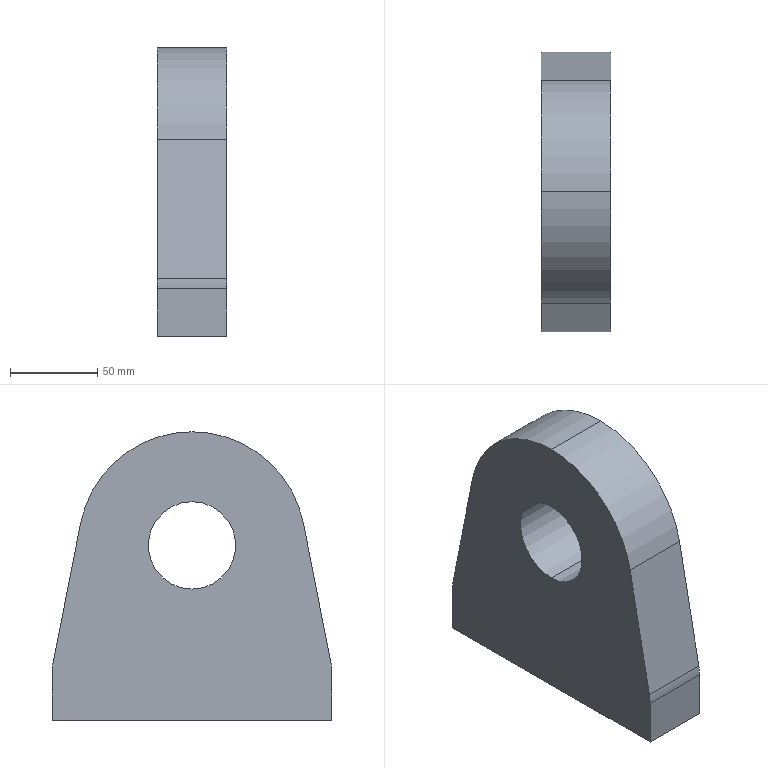Part | SolidWorks | features BaseBody 1 | 1 solid | 13 faces | box 40 x 160 x 165 mm | volume 788802 mm3 | plane 7 | cylinder 6 | commonest cylinder face diameters 50 x2 60 x2 130 x2
STEP:
#1=CARTESIAN_POINT('',(20.,0.,42.5));
#2=VERTEX_POINT('',#1);
#3=CARTESIAN_POINT('',(20.,0.,-7.5));
#4=VERTEX_POINT('',#3);
#5=CARTESIAN_POINT('',(20.,0.,17.5));
#6=DIRECTION('',(1.,0.,0.));
#7=DIRECTION('',(0.,0.,-1.));
#8=AXIS2_PLACEMENT_3D('',#5,#6,#7);
#9=CIRCLE('',#8,25.);
#10=EDGE_CURVE('',#2,#4,#9,.T.);
#11=ORIENTED_EDGE('',*,*,#10,.T.);
#12=CARTESIAN_POINT('',(-20.,0.,-7.5));
#13=VERTEX_POINT('',#12);
#14=CARTESIAN_POINT('',(20.,0.,-7.5));
#15=DIRECTION('',(-1.,0.,0.));
#16=VECTOR('',#15,1000.);
#17=LINE('',#14,#16);
#18=EDGE_CURVE('',#4,#13,#17,.T.);
#19=ORIENTED_EDGE('',*,*,#18,.T.);
#20=CARTESIAN_POINT('',(-20.,0.,42.5));
#21=VERTEX_POINT('',#20);
#22=CARTESIAN_POINT('',(-20.,0.,17.5));
#23=DIRECTION('',(1.,0.,0.));
#24=DIRECTION('',(0.,0.,-1.));
#25=AXIS2_PLACEMENT_3D('',#22,#23,#24);
#26=CIRCLE('',#25,25.);
#27=EDGE_CURVE('',#21,#13,#26,.T.);
#28=ORIENTED_EDGE('',*,*,#27,.F.);
#29=CARTESIAN_POINT('',(20.,0.,42.5));
#30=DIRECTION('',(-1.,0.,0.));
#31=VECTOR('',#30,1000.);
#32=LINE('',#29,#31);
#33=EDGE_CURVE('',#2,#21,#32,.T.);
#34=ORIENTED_EDGE('',*,*,#33,.F.);
#35=EDGE_LOOP('',(#11,#19,#28,#34));
#36=FACE_OUTER_BOUND('',#35,.T.);
#37=CARTESIAN_POINT('',(20.,0.,17.5));
#38=DIRECTION('',(-1.,0.,0.));
#39=DIRECTION('',(0.,0.,1.));
#40=AXIS2_PLACEMENT_3D('',#37,#38,#39);
#41=CYLINDRICAL_SURFACE('',#40,25.);
#42=ADVANCED_FACE('',(#36),#41,.F.);
#43=CARTESIAN_POINT('',(20.,0.,82.5));
#44=VERTEX_POINT('',#43);
#45=CARTESIAN_POINT('',(20.,-63.78,30.034));
#46=VERTEX_POINT('',#45);
#47=CARTESIAN_POINT('',(20.,0.,17.5));
#48=DIRECTION('',(1.,0.,0.));
#49=DIRECTION('',(0.,0.,-1.));
#50=AXIS2_PLACEMENT_3D('',#47,#48,#49);
#51=CIRCLE('',#50,65.);
#52=EDGE_CURVE('',#44,#46,#51,.T.);
#53=ORIENTED_EDGE('',*,*,#52,.F.);
#54=CARTESIAN_POINT('',(-20.,0.,82.5));
#55=VERTEX_POINT('',#54);
#56=CARTESIAN_POINT('',(20.,0.,82.5));
#57=DIRECTION('',(-1.,0.,0.));
#58=VECTOR('',#57,1000.);
#59=LINE('',#56,#58);
#60=EDGE_CURVE('',#44,#55,#59,.T.);
#61=ORIENTED_EDGE('',*,*,#60,.T.);
#62=CARTESIAN_POINT('',(-20.,-63.78,30.034));
#63=VERTEX_POINT('',#62);
#64=CARTESIAN_POINT('',(-20.,0.,17.5));
#65=DIRECTION('',(1.,0.,0.));
#66=DIRECTION('',(0.,0.,-1.));
#67=AXIS2_PLACEMENT_3D('',#64,#65,#66);
#68=CIRCLE('',#67,65.);
#69=EDGE_CURVE('',#55,#63,#68,.T.);
#70=ORIENTED_EDGE('',*,*,#69,.T.);
#71=CARTESIAN_POINT('',(20.,-63.78,30.034));
#72=DIRECTION('',(-1.,0.,0.));
#73=VECTOR('',#72,1000.);
#74=LINE('',#71,#73);
#75=EDGE_CURVE('',#46,#63,#74,.T.);
#76=ORIENTED_EDGE('',*,*,#75,.F.);
#77=EDGE_LOOP('',(#53,#61,#70,#76));
#78=FACE_OUTER_BOUND('',#77,.T.);
#79=CARTESIAN_POINT('',(20.,0.,17.5));
#80=DIRECTION('',(-1.,0.,0.));
#81=DIRECTION('',(0.,0.,1.));
#82=AXIS2_PLACEMENT_3D('',#79,#80,#81);
#83=CYLINDRICAL_SURFACE('',#82,65.);
#84=ADVANCED_FACE('',(#78),#83,.T.);
#85=CARTESIAN_POINT('',(20.,80.,-82.5));
#86=VERTEX_POINT('',#85);
#87=CARTESIAN_POINT('',(20.,80.,-55.42));
#88=VERTEX_POINT('',#87);
#89=CARTESIAN_POINT('',(20.,80.,-82.5));
#90=DIRECTION('',(0.,0.,1.));
#91=VECTOR('',#90,1000.);
#92=LINE('',#89,#91);
#93=EDGE_CURVE('',#86,#88,#92,.T.);
#94=ORIENTED_EDGE('',*,*,#93,.T.);
#95=CARTESIAN_POINT('',(20.,79.437,-49.635));
#96=VERTEX_POINT('',#95);
#97=CARTESIAN_POINT('',(20.,50.,-55.42));
#98=DIRECTION('',(1.,0.,0.));
#99=DIRECTION('',(0.,0.,1.));
#100=AXIS2_PLACEMENT_3D('',#97,#98,#99);
#101=CIRCLE('',#100,30.);
#102=EDGE_CURVE('',#88,#96,#101,.T.);
#103=ORIENTED_EDGE('',*,*,#102,.T.);
#104=CARTESIAN_POINT('',(20.,63.78,30.034));
#105=VERTEX_POINT('',#104);
#106=CARTESIAN_POINT('',(20.,79.437,-49.635));
#107=DIRECTION('',(0.,-0.1928,0.9812));
#108=VECTOR('',#107,1000.);
#109=LINE('',#106,#108);
#110=EDGE_CURVE('',#96,#105,#109,.T.);
#111=ORIENTED_EDGE('',*,*,#110,.T.);
#112=CARTESIAN_POINT('',(20.,0.,17.5));
#113=DIRECTION('',(1.,0.,0.));
#114=DIRECTION('',(0.,0.,-1.));
#115=AXIS2_PLACEMENT_3D('',#112,#113,#114);
#116=CIRCLE('',#115,65.);
#117=EDGE_CURVE('',#105,#44,#116,.T.);
#118=ORIENTED_EDGE('',*,*,#117,.T.);
#119=ORIENTED_EDGE('',*,*,#52,.T.);
#120=CARTESIAN_POINT('',(20.,-79.437,-49.635));
#121=VERTEX_POINT('',#120);
#122=CARTESIAN_POINT('',(20.,-79.437,-49.635));
#123=DIRECTION('',(0.,-0.1928,-0.9812));
#124=VECTOR('',#123,1000.);
#125=LINE('',#122,#124);
#126=EDGE_CURVE('',#46,#121,#125,.T.);
#127=ORIENTED_EDGE('',*,*,#126,.T.);
#128=CARTESIAN_POINT('',(20.,-80.,-55.42));
#129=VERTEX_POINT('',#128);
#130=CARTESIAN_POINT('',(20.,-50.,-55.42));
#131=DIRECTION('',(1.,0.,0.));
#132=DIRECTION('',(0.,0.,-1.));
#133=AXIS2_PLACEMENT_3D('',#130,#131,#132);
#134=CIRCLE('',#133,30.);
#135=EDGE_CURVE('',#121,#129,#134,.T.);
#136=ORIENTED_EDGE('',*,*,#135,.T.);
#137=CARTESIAN_POINT('',(20.,-80.,-82.5));
#138=VERTEX_POINT('',#137);
#139=CARTESIAN_POINT('',(20.,-80.,-82.5));
#140=DIRECTION('',(0.,0.,-1.));
#141=VECTOR('',#140,1000.);
#142=LINE('',#139,#141);
#143=EDGE_CURVE('',#129,#138,#142,.T.);
#144=ORIENTED_EDGE('',*,*,#143,.T.);
#145=CARTESIAN_POINT('',(20.,80.,-82.5));
#146=DIRECTION('',(0.,1.,0.));
#147=VECTOR('',#146,1000.);
#148=LINE('',#145,#147);
#149=EDGE_CURVE('',#138,#86,#148,.T.);
#150=ORIENTED_EDGE('',*,*,#149,.T.);
#151=EDGE_LOOP('',(#94,#103,#111,#118,#119,#127,#136,#144,#150));
#152=FACE_OUTER_BOUND('',#151,.T.);
#153=ORIENTED_EDGE('',*,*,#10,.F.);
#154=CARTESIAN_POINT('',(20.,0.,17.5));
#155=DIRECTION('',(1.,0.,0.));
#156=DIRECTION('',(0.,0.,-1.));
#157=AXIS2_PLACEMENT_3D('',#154,#155,#156);
#158=CIRCLE('',#157,25.);
#159=EDGE_CURVE('',#4,#2,#158,.T.);
#160=ORIENTED_EDGE('',*,*,#159,.F.);
#161=EDGE_LOOP('',(#153,#160));
#162=FACE_BOUND('',#161,.T.);
#163=CARTESIAN_POINT('',(20.,50.,-55.42));
#164=DIRECTION('',(-1.,0.,0.));
#165=DIRECTION('',(0.,0.,1.));
#166=AXIS2_PLACEMENT_3D('',#163,#164,#165);
#167=PLANE('',#166);
#168=ADVANCED_FACE('',(#152,#162),#167,.F.);
#169=CARTESIAN_POINT('',(-20.,80.,-82.5));
#170=VERTEX_POINT('',#169);
#171=CARTESIAN_POINT('',(-20.,80.,-55.42));
#172=VERTEX_POINT('',#171);
#173=CARTESIAN_POINT('',(-20.,80.,-82.5));
#174=DIRECTION('',(0.,0.,1.));
#175=VECTOR('',#174,1000.);
#176=LINE('',#173,#175);
#177=EDGE_CURVE('',#170,#172,#176,.T.);
#178=ORIENTED_EDGE('',*,*,#177,.F.);
#179=CARTESIAN_POINT('',(-20.,-80.,-82.5));
#180=VERTEX_POINT('',#179);
#181=CARTESIAN_POINT('',(-20.,80.,-82.5));
#182=DIRECTION('',(0.,1.,0.));
#183=VECTOR('',#182,1000.);
#184=LINE('',#181,#183);
#185=EDGE_CURVE('',#180,#170,#184,.T.);
#186=ORIENTED_EDGE('',*,*,#185,.F.);
#187=CARTESIAN_POINT('',(-20.,-80.,-55.42));
#188=VERTEX_POINT('',#187);
#189=CARTESIAN_POINT('',(-20.,-80.,-82.5));
#190=DIRECTION('',(0.,0.,-1.));
#191=VECTOR('',#190,1000.);
#192=LINE('',#189,#191);
#193=EDGE_CURVE('',#188,#180,#192,.T.);
#194=ORIENTED_EDGE('',*,*,#193,.F.);
#195=CARTESIAN_POINT('',(-20.,-79.437,-49.635));
#196=VERTEX_POINT('',#195);
#197=CARTESIAN_POINT('',(-20.,-50.,-55.42));
#198=DIRECTION('',(1.,0.,0.));
#199=DIRECTION('',(0.,0.,-1.));
#200=AXIS2_PLACEMENT_3D('',#197,#198,#199);
#201=CIRCLE('',#200,30.);
#202=EDGE_CURVE('',#196,#188,#201,.T.);
#203=ORIENTED_EDGE('',*,*,#202,.F.);
#204=CARTESIAN_POINT('',(-20.,-79.437,-49.635));
#205=DIRECTION('',(0.,-0.1928,-0.9812));
#206=VECTOR('',#205,1000.);
#207=LINE('',#204,#206);
#208=EDGE_CURVE('',#63,#196,#207,.T.);
#209=ORIENTED_EDGE('',*,*,#208,.F.);
#210=ORIENTED_EDGE('',*,*,#69,.F.);
#211=CARTESIAN_POINT('',(-20.,63.78,30.034));
#212=VERTEX_POINT('',#211);
#213=CARTESIAN_POINT('',(-20.,0.,17.5));
#214=DIRECTION('',(1.,0.,0.));
#215=DIRECTION('',(0.,0.,-1.));
#216=AXIS2_PLACEMENT_3D('',#213,#214,#215);
#217=CIRCLE('',#216,65.);
#218=EDGE_CURVE('',#212,#55,#217,.T.);
#219=ORIENTED_EDGE('',*,*,#218,.F.);
#220=CARTESIAN_POINT('',(-20.,79.437,-49.635));
#221=VERTEX_POINT('',#220);
#222=CARTESIAN_POINT('',(-20.,79.437,-49.635));
#223=DIRECTION('',(0.,-0.1928,0.9812));
#224=VECTOR('',#223,1000.);
#225=LINE('',#222,#224);
#226=EDGE_CURVE('',#221,#212,#225,.T.);
#227=ORIENTED_EDGE('',*,*,#226,.F.);
#228=CARTESIAN_POINT('',(-20.,50.,-55.42));
#229=DIRECTION('',(1.,0.,0.));
#230=DIRECTION('',(0.,0.,1.));
#231=AXIS2_PLACEMENT_3D('',#228,#229,#230);
#232=CIRCLE('',#231,30.);
#233=EDGE_CURVE('',#172,#221,#232,.T.);
#234=ORIENTED_EDGE('',*,*,#233,.F.);
#235=EDGE_LOOP('',(#178,#186,#194,#203,#209,#210,#219,#227,#234));
#236=FACE_OUTER_BOUND('',#235,.T.);
#237=ORIENTED_EDGE('',*,*,#27,.T.);
#238=CARTESIAN_POINT('',(-20.,0.,17.5));
#239=DIRECTION('',(1.,0.,0.));
#240=DIRECTION('',(0.,0.,-1.));
#241=AXIS2_PLACEMENT_3D('',#238,#239,#240);
#242=CIRCLE('',#241,25.);
#243=EDGE_CURVE('',#13,#21,#242,.T.);
#244=ORIENTED_EDGE('',*,*,#243,.T.);
#245=EDGE_LOOP('',(#237,#244));
#246=FACE_BOUND('',#245,.T.);
#247=CARTESIAN_POINT('',(-20.,50.,-55.42));
#248=DIRECTION('',(-1.,0.,0.));
#249=DIRECTION('',(0.,0.,1.));
#250=AXIS2_PLACEMENT_3D('',#247,#248,#249);
#251=PLANE('',#250);
#252=ADVANCED_FACE('',(#236,#246),#251,.T.);
#253=ORIENTED_EDGE('',*,*,#177,.T.);
#254=CARTESIAN_POINT('',(20.,80.,-55.42));
#255=DIRECTION('',(-1.,0.,0.));
#256=VECTOR('',#255,1000.);
#257=LINE('',#254,#256);
#258=EDGE_CURVE('',#88,#172,#257,.T.);
#259=ORIENTED_EDGE('',*,*,#258,.F.);
#260=ORIENTED_EDGE('',*,*,#93,.F.);
#261=CARTESIAN_POINT('',(20.,80.,-82.5));
#262=DIRECTION('',(-1.,0.,0.));
#263=VECTOR('',#262,1000.);
#264=LINE('',#261,#263);
#265=EDGE_CURVE('',#86,#170,#264,.T.);
#266=ORIENTED_EDGE('',*,*,#265,.T.);
#267=EDGE_LOOP('',(#253,#259,#260,#266));
#268=FACE_OUTER_BOUND('',#267,.T.);
#269=CARTESIAN_POINT('',(20.,80.,-82.5));
#270=DIRECTION('',(0.,-1.,0.));
#271=DIRECTION('',(0.,0.,-1.));
#272=AXIS2_PLACEMENT_3D('',#269,#270,#271);
#273=PLANE('',#272);
#274=ADVANCED_FACE('',(#268),#273,.F.);
#275=ORIENTED_EDGE('',*,*,#233,.T.);
#276=CARTESIAN_POINT('',(20.,79.437,-49.635));
#277=DIRECTION('',(-1.,0.,0.));
#278=VECTOR('',#277,1000.);
#279=LINE('',#276,#278);
#280=EDGE_CURVE('',#96,#221,#279,.T.);
#281=ORIENTED_EDGE('',*,*,#280,.F.);
#282=ORIENTED_EDGE('',*,*,#102,.F.);
#283=ORIENTED_EDGE('',*,*,#258,.T.);
#284=EDGE_LOOP('',(#275,#281,#282,#283));
#285=FACE_OUTER_BOUND('',#284,.T.);
#286=CARTESIAN_POINT('',(20.,50.,-55.42));
#287=DIRECTION('',(-1.,0.,0.));
#288=DIRECTION('',(0.,0.,1.));
#289=AXIS2_PLACEMENT_3D('',#286,#287,#288);
#290=CYLINDRICAL_SURFACE('',#289,30.);
#291=ADVANCED_FACE('',(#285),#290,.T.);
#292=ORIENTED_EDGE('',*,*,#226,.T.);
#293=CARTESIAN_POINT('',(20.,63.78,30.034));
#294=DIRECTION('',(-1.,0.,0.));
#295=VECTOR('',#294,1000.);
#296=LINE('',#293,#295);
#297=EDGE_CURVE('',#105,#212,#296,.T.);
#298=ORIENTED_EDGE('',*,*,#297,.F.);
#299=ORIENTED_EDGE('',*,*,#110,.F.);
#300=ORIENTED_EDGE('',*,*,#280,.T.);
#301=EDGE_LOOP('',(#292,#298,#299,#300));
#302=FACE_OUTER_BOUND('',#301,.T.);
#303=CARTESIAN_POINT('',(20.,79.437,-49.635));
#304=DIRECTION('',(0.,-0.9812,-0.1928));
#305=DIRECTION('',(0.,0.1928,-0.9812));
#306=AXIS2_PLACEMENT_3D('',#303,#304,#305);
#307=PLANE('',#306);
#308=ADVANCED_FACE('',(#302),#307,.F.);
#309=ORIENTED_EDGE('',*,*,#60,.F.);
#310=ORIENTED_EDGE('',*,*,#117,.F.);
#311=ORIENTED_EDGE('',*,*,#297,.T.);
#312=ORIENTED_EDGE('',*,*,#218,.T.);
#313=EDGE_LOOP('',(#309,#310,#311,#312));
#314=FACE_OUTER_BOUND('',#313,.T.);
#315=CARTESIAN_POINT('',(20.,0.,17.5));
#316=DIRECTION('',(-1.,0.,0.));
#317=DIRECTION('',(0.,0.,1.));
#318=AXIS2_PLACEMENT_3D('',#315,#316,#317);
#319=CYLINDRICAL_SURFACE('',#318,65.);
#320=ADVANCED_FACE('',(#314),#319,.T.);
#321=ORIENTED_EDGE('',*,*,#208,.T.);
#322=CARTESIAN_POINT('',(20.,-79.437,-49.635));
#323=DIRECTION('',(-1.,0.,0.));
#324=VECTOR('',#323,1000.);
#325=LINE('',#322,#324);
#326=EDGE_CURVE('',#121,#196,#325,.T.);
#327=ORIENTED_EDGE('',*,*,#326,.F.);
#328=ORIENTED_EDGE('',*,*,#126,.F.);
#329=ORIENTED_EDGE('',*,*,#75,.T.);
#330=EDGE_LOOP('',(#321,#327,#328,#329));
#331=FACE_OUTER_BOUND('',#330,.T.);
#332=CARTESIAN_POINT('',(20.,-79.437,-49.635));
#333=DIRECTION('',(0.,0.9812,-0.1928));
#334=DIRECTION('',(0.,0.1928,0.9812));
#335=AXIS2_PLACEMENT_3D('',#332,#333,#334);
#336=PLANE('',#335);
#337=ADVANCED_FACE('',(#331),#336,.F.);
#338=ORIENTED_EDGE('',*,*,#202,.T.);
#339=CARTESIAN_POINT('',(20.,-80.,-55.42));
#340=DIRECTION('',(-1.,0.,0.));
#341=VECTOR('',#340,1000.);
#342=LINE('',#339,#341);
#343=EDGE_CURVE('',#129,#188,#342,.T.);
#344=ORIENTED_EDGE('',*,*,#343,.F.);
#345=ORIENTED_EDGE('',*,*,#135,.F.);
#346=ORIENTED_EDGE('',*,*,#326,.T.);
#347=EDGE_LOOP('',(#338,#344,#345,#346));
#348=FACE_OUTER_BOUND('',#347,.T.);
#349=CARTESIAN_POINT('',(20.,-50.,-55.42));
#350=DIRECTION('',(-1.,0.,0.));
#351=DIRECTION('',(0.,0.,1.));
#352=AXIS2_PLACEMENT_3D('',#349,#350,#351);
#353=CYLINDRICAL_SURFACE('',#352,30.);
#354=ADVANCED_FACE('',(#348),#353,.T.);
#355=ORIENTED_EDGE('',*,*,#193,.T.);
#356=CARTESIAN_POINT('',(20.,-80.,-82.5));
#357=DIRECTION('',(-1.,0.,0.));
#358=VECTOR('',#357,1000.);
#359=LINE('',#356,#358);
#360=EDGE_CURVE('',#138,#180,#359,.T.);
#361=ORIENTED_EDGE('',*,*,#360,.F.);
#362=ORIENTED_EDGE('',*,*,#143,.F.);
#363=ORIENTED_EDGE('',*,*,#343,.T.);
#364=EDGE_LOOP('',(#355,#361,#362,#363));
#365=FACE_OUTER_BOUND('',#364,.T.);
#366=CARTESIAN_POINT('',(20.,-80.,-82.5));
#367=DIRECTION('',(0.,1.,0.));
#368=DIRECTION('',(0.,0.,1.));
#369=AXIS2_PLACEMENT_3D('',#366,#367,#368);
#370=PLANE('',#369);
#371=ADVANCED_FACE('',(#365),#370,.F.);
#372=ORIENTED_EDGE('',*,*,#185,.T.);
#373=ORIENTED_EDGE('',*,*,#265,.F.);
#374=ORIENTED_EDGE('',*,*,#149,.F.);
#375=ORIENTED_EDGE('',*,*,#360,.T.);
#376=EDGE_LOOP('',(#372,#373,#374,#375));
#377=FACE_OUTER_BOUND('',#376,.T.);
#378=CARTESIAN_POINT('',(20.,80.,-82.5));
#379=DIRECTION('',(0.,0.,1.));
#380=DIRECTION('',(1.,0.,0.));
#381=AXIS2_PLACEMENT_3D('',#378,#379,#380);
#382=PLANE('',#381);
#383=ADVANCED_FACE('',(#377),#382,.F.);
#384=ORIENTED_EDGE('',*,*,#18,.F.);
#385=ORIENTED_EDGE('',*,*,#159,.T.);
#386=ORIENTED_EDGE('',*,*,#33,.T.);
#387=ORIENTED_EDGE('',*,*,#243,.F.);
#388=EDGE_LOOP('',(#384,#385,#386,#387));
#389=FACE_OUTER_BOUND('',#388,.T.);
#390=CARTESIAN_POINT('',(20.,0.,17.5));
#391=DIRECTION('',(-1.,0.,0.));
#392=DIRECTION('',(0.,0.,1.));
#393=AXIS2_PLACEMENT_3D('',#390,#391,#392);
#394=CYLINDRICAL_SURFACE('',#393,25.);
#395=ADVANCED_FACE('',(#389),#394,.F.);
#396=CLOSED_SHELL('',(#42,#84,#168,#252,#274,#291,#308,#320,#337,#354,#371,#383,#395));
#397=MANIFOLD_SOLID_BREP('',#396);
#398=CARTESIAN_POINT('',(0.,0.,0.));
#399=DIRECTION('',(0.,0.,1.));
#400=DIRECTION('',(1.,0.,0.));
#401=AXIS2_PLACEMENT_3D('',#398,#399,#400);
#402=(LENGTH_UNIT()NAMED_UNIT(*)SI_UNIT(.MILLI.,.METRE.));
#403=UNCERTAINTY_MEASURE_WITH_UNIT(LENGTH_MEASURE(0.00001),#402,'','');
#404=(NAMED_UNIT(*)PLANE_ANGLE_UNIT()SI_UNIT($,.RADIAN.));
#405=(NAMED_UNIT(*)SI_UNIT($,.STERADIAN.)SOLID_ANGLE_UNIT());
#406=(GEOMETRIC_REPRESENTATION_CONTEXT(3)GLOBAL_UNCERTAINTY_ASSIGNED_CONTEXT((#403))GLOBAL_UNIT_ASSIGNED_CONTEXT((#402,#404,#405))REPRESENTATION_CONTEXT('',''));
#407=ADVANCED_BREP_SHAPE_REPRESENTATION('',(#397,#401),#406);